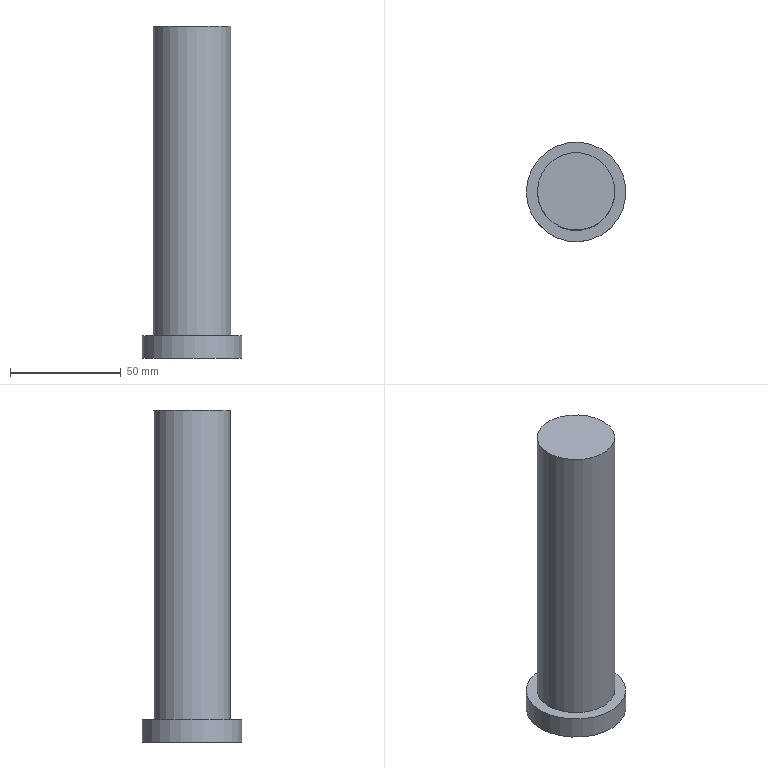Part | NX | features 护邦千斤顶活塞销 2 | 1 solid | 5 faces | box 45 x 45 x 150 mm | volume 150600 mm3 | plane 3 | cylinder 2 | commonest cylinder face diameters 35 x1 45 x1
STEP:
#1=CARTESIAN_POINT('',(17.5,0.,140.));
#2=VERTEX_POINT('',#1);
#3=CARTESIAN_POINT('',(0.,0.,140.));
#4=DIRECTION('',(0.,0.,1.));
#5=DIRECTION('',(1.,0.,0.));
#6=AXIS2_PLACEMENT_3D('',#3,#4,#5);
#7=CIRCLE('',#6,17.5);
#8=EDGE_CURVE('',#2,#2,#7,.T.);
#9=ORIENTED_EDGE('',*,*,#8,.F.);
#10=EDGE_LOOP('',(#9));
#11=FACE_BOUND('',#10,.T.);
#12=CARTESIAN_POINT('',(-17.5,0.,0.));
#13=VERTEX_POINT('',#12);
#14=CARTESIAN_POINT('',(0.,0.,0.));
#15=DIRECTION('',(0.,0.,-1.));
#16=DIRECTION('',(-1.,0.,0.));
#17=AXIS2_PLACEMENT_3D('',#14,#15,#16);
#18=CIRCLE('',#17,17.5);
#19=EDGE_CURVE('',#13,#13,#18,.T.);
#20=ORIENTED_EDGE('',*,*,#19,.F.);
#21=EDGE_LOOP('',(#20));
#22=FACE_BOUND('',#21,.T.);
#23=CARTESIAN_POINT('',(0.,0.,140.));
#24=DIRECTION('',(0.,0.,-1.));
#25=DIRECTION('',(-1.,0.,0.));
#26=AXIS2_PLACEMENT_3D('',#23,#24,#25);
#27=CYLINDRICAL_SURFACE('',#26,17.5);
#28=ADVANCED_FACE('',(#11,#22),#27,.T.);
#29=ORIENTED_EDGE('',*,*,#8,.T.);
#30=EDGE_LOOP('',(#29));
#31=FACE_BOUND('',#30,.T.);
#32=CARTESIAN_POINT('',(0.,0.,140.));
#33=DIRECTION('',(0.,0.,1.));
#34=DIRECTION('',(1.,0.,0.));
#35=AXIS2_PLACEMENT_3D('',#32,#33,#34);
#36=PLANE('',#35);
#37=ADVANCED_FACE('',(#31),#36,.T.);
#38=CARTESIAN_POINT('',(-22.5,0.,0.));
#39=VERTEX_POINT('',#38);
#40=CARTESIAN_POINT('',(0.,0.,0.));
#41=DIRECTION('',(0.,0.,-1.));
#42=DIRECTION('',(-1.,0.,0.));
#43=AXIS2_PLACEMENT_3D('',#40,#41,#42);
#44=CIRCLE('',#43,22.5);
#45=EDGE_CURVE('',#39,#39,#44,.T.);
#46=ORIENTED_EDGE('',*,*,#45,.F.);
#47=EDGE_LOOP('',(#46));
#48=FACE_BOUND('',#47,.T.);
#49=ORIENTED_EDGE('',*,*,#19,.T.);
#50=EDGE_LOOP('',(#49));
#51=FACE_BOUND('',#50,.T.);
#52=CARTESIAN_POINT('',(0.,0.,0.));
#53=DIRECTION('',(0.,0.,-1.));
#54=DIRECTION('',(-1.,0.,0.));
#55=AXIS2_PLACEMENT_3D('',#52,#53,#54);
#56=PLANE('',#55);
#57=ADVANCED_FACE('',(#48,#51),#56,.F.);
#58=CARTESIAN_POINT('',(-22.5,0.,-10.));
#59=VERTEX_POINT('',#58);
#60=CARTESIAN_POINT('',(0.,0.,-10.));
#61=DIRECTION('',(0.,0.,-1.));
#62=DIRECTION('',(-1.,0.,0.));
#63=AXIS2_PLACEMENT_3D('',#60,#61,#62);
#64=CIRCLE('',#63,22.5);
#65=EDGE_CURVE('',#59,#59,#64,.T.);
#66=ORIENTED_EDGE('',*,*,#65,.F.);
#67=EDGE_LOOP('',(#66));
#68=FACE_BOUND('',#67,.T.);
#69=ORIENTED_EDGE('',*,*,#45,.T.);
#70=EDGE_LOOP('',(#69));
#71=FACE_BOUND('',#70,.T.);
#72=CARTESIAN_POINT('',(0.,0.,-10.));
#73=DIRECTION('',(0.,0.,1.));
#74=DIRECTION('',(1.,0.,0.));
#75=AXIS2_PLACEMENT_3D('',#72,#73,#74);
#76=CYLINDRICAL_SURFACE('',#75,22.5);
#77=ADVANCED_FACE('',(#68,#71),#76,.T.);
#78=ORIENTED_EDGE('',*,*,#65,.T.);
#79=EDGE_LOOP('',(#78));
#80=FACE_BOUND('',#79,.T.);
#81=CARTESIAN_POINT('',(0.,0.,-10.));
#82=DIRECTION('',(0.,0.,-1.));
#83=DIRECTION('',(-1.,0.,0.));
#84=AXIS2_PLACEMENT_3D('',#81,#82,#83);
#85=PLANE('',#84);
#86=ADVANCED_FACE('',(#80),#85,.T.);
#87=CLOSED_SHELL('',(#28,#37,#57,#77,#86));
#88=MANIFOLD_SOLID_BREP('',#87);
#89=(LENGTH_UNIT()NAMED_UNIT(*)SI_UNIT(.MILLI.,.METRE.));
#90=UNCERTAINTY_MEASURE_WITH_UNIT(LENGTH_MEASURE(0.00001),#89,'','');
#91=(NAMED_UNIT(*)PLANE_ANGLE_UNIT()SI_UNIT($,.RADIAN.));
#92=(NAMED_UNIT(*)SI_UNIT($,.STERADIAN.)SOLID_ANGLE_UNIT());
#93=(GEOMETRIC_REPRESENTATION_CONTEXT(3)GLOBAL_UNCERTAINTY_ASSIGNED_CONTEXT((#90))GLOBAL_UNIT_ASSIGNED_CONTEXT((#89,#91,#92))REPRESENTATION_CONTEXT('',''));
#94=ADVANCED_BREP_SHAPE_REPRESENTATION('',(#88),#93);